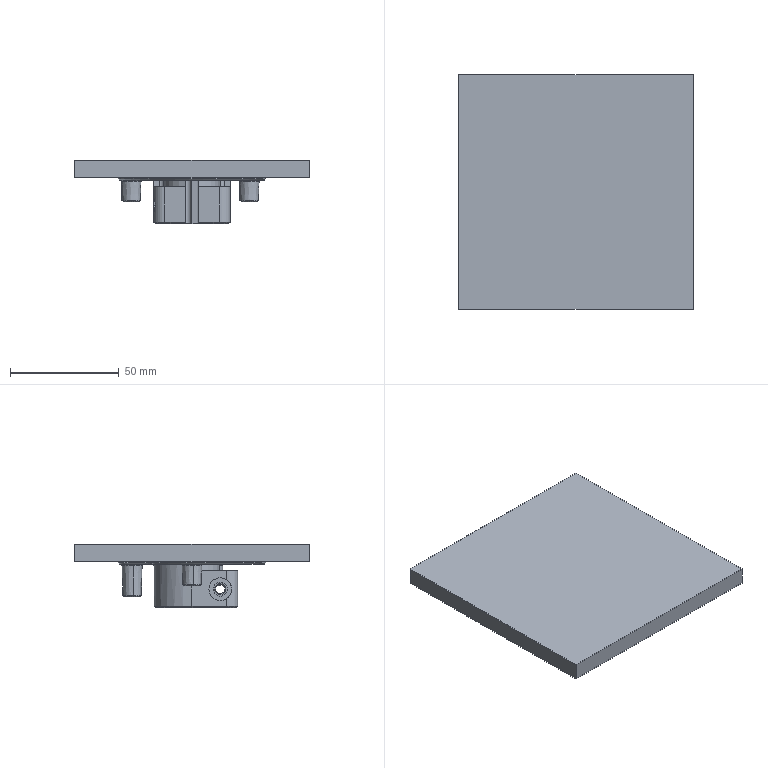NC program | NX | posted with a generic post | part box 108 x 108 x 29 mm
Lines 5403 to 6183 of 23883:
(ZLEVEL_PROFILE_COPY_COPY_COPY_COPY_1 , TOOL : D3R0.5)
N10768 T07 M6
N10770 G54
N10772 G17 G0 G90 X-0.847 Y24.584 S9500 M3
N10774 G43 Z30. H7
N10776 Z-4.
N10778 G94 G1 X-1.263 Y24.078 Z-4.034 F1000.
N10780 X-1.883 Y23.537 Z-4.077
N10782 X-2.582 Y23.105 Z-4.121
N10784 X-3.342 Y22.793 Z-4.164
N10786 X-4.144 Y22.608 Z-4.207
N10788 X-4.964 Y22.558 Z-4.25
N10790 X-5.782 Y22.642 Z-4.293
N10792 X-6.575 Y22.858 Z-4.336
N10794 X-7.322 Y23.201 Z-4.379
N10796 X-8.003 Y23.661 Z-4.422
N10798 X-8.6 Y24.227 Z-4.465
N10800 X-8.992 Y24.724 Z-4.498
N10802 X-9.402 Y25.437 Z-4.541
N10804 X-9.691 Y26.206 Z-4.585
N10806 X-9.849 Y27.013 Z-4.628
N10808 X-9.874 Y27.835 Z-4.671
N10810 X-9.764 Y28.65 Z-4.714
N10812 X-9.523 Y29.436 Z-4.757
N10814 X-9.157 Y30.172 Z-4.8
N10816 X-8.675 Y30.838 Z-4.843
N10818 X-8.091 Y31.417 Z-4.886
N10820 X-7.421 Y31.892 Z-4.929
N10822 X-6.681 Y32.252 Z-4.972
N10824 X-5.893 Y32.486 Z-5.015
N10826 X-5.267 Y32.577 Z-5.049
N10828 X-5.179 Y32.583 Z-5.053
N10830 X-4.863 Z-5.07
N10832 G2 X0.146 Y27.575 R5.008 F2000.
N10834 X-4.863 Y32.583 R-5.008
N10836 G1 X-4.745 Y32.579 Z-5.072
N10838 X-4.627 Y32.577 Z-5.074
N10840 X-4.51 Y32.575 Z-5.076
N10842 X-4.392 Y32.573 Z-5.078
N10844 X-4.274 Y32.563 Z-5.08
N10846 X-4.158 Y32.545 Z-5.082
N10848 X-4.041 Y32.53 Z-5.084
N10850 X-3.924 Y32.513 Z-5.086
N10852 X-3.808 Y32.492 Z-5.088
N10854 X-3.691 Y32.472 Z-5.09
N10856 X-3.576 Y32.444 Z-5.092
N10858 X-3.462 Y32.414 Z-5.094
N10860 X-3.348 Y32.383 Z-5.096
N10862 X-3.235 Y32.348 Z-5.099
N10864 X-3.122 Y32.311 Z-5.101
N10866 X-3.01 Y32.273 Z-5.103
N10868 X-2.899 Y32.229 Z-5.105
N10870 X-2.79 Y32.185 Z-5.107
N10872 X-2.681 Y32.137 Z-5.109
N10874 X-2.573 Y32.087 Z-5.111
N10876 X-2.467 Y32.034 Z-5.113
N10878 X-2.361 Y31.979 Z-5.115
N10880 X-2.258 Y31.921 Z-5.117
N10882 X-2.155 Y31.861 Z-5.119
N10884 X-2.054 Y31.798 Z-5.121
N10886 X-1.954 Y31.733 Z-5.123
N10888 X-1.856 Y31.665 Z-5.125
N10890 X-1.759 Y31.595 Z-5.127
N10892 X-1.664 Y31.523 Z-5.129
N10894 X-1.571 Y31.449 Z-5.131
N10896 X-1.479 Y31.372 Z-5.133
N10898 X-1.39 Y31.293 Z-5.135
N10900 X-1.302 Y31.212 Z-5.138
N10902 X-1.216 Y31.129 Z-5.14
N10904 G2 X-4.863 Y32.667 R-5.092
N10906 G1 X-4.745 Y32.668 Z-5.142
N10908 X-4.627 Y32.666 Z-5.144
N10910 X-4.51 Y32.661 Z-5.146
N10912 X-4.392 Y32.653 Z-5.148
N10914 X-4.275 Y32.643 Z-5.15
N10916 X-4.158 Y32.631 Z-5.152
N10918 X-4.041 Y32.615 Z-5.154
N10920 X-3.924 Y32.597 Z-5.156
N10922 X-3.808 Y32.576 Z-5.158
N10924 X-3.692 Y32.552 Z-5.16
N10926 X-3.577 Y32.526 Z-5.162
N10928 X-3.463 Y32.497 Z-5.164
N10930 X-3.349 Y32.465 Z-5.166
N10932 X-3.236 Y32.431 Z-5.168
N10934 X-3.123 Y32.394 Z-5.17
N10936 X-3.012 Y32.355 Z-5.172
N10938 X-2.901 Y32.313 Z-5.174
N10940 X-2.791 Y32.268 Z-5.177
N10942 X-2.682 Y32.221 Z-5.179
N10944 X-2.575 Y32.171 Z-5.181
N10946 X-2.468 Y32.119 Z-5.183
N10948 X-2.363 Y32.064 Z-5.185
N10950 X-2.259 Y32.007 Z-5.187
N10952 X-2.156 Y31.948 Z-5.189
N10954 X-2.055 Y31.886 Z-5.191
N10956 X-1.955 Y31.822 Z-5.193
N10958 X-1.856 Y31.755 Z-5.195
N10960 X-1.759 Y31.686 Z-5.197
N10962 X-1.664 Y31.615 Z-5.199
N10964 X-1.57 Y31.542 Z-5.201
N10966 X-1.478 Y31.467 Z-5.203
N10968 X-1.388 Y31.389 Z-5.205
N10970 X-1.299 Y31.309 Z-5.207
N10972 X-1.212 Y31.227 Z-5.209
N10974 G2 X-4.863 Y32.738 R-5.164
N10976 G1 X-4.745 Y32.739 Z-5.211
N10978 X-4.627 Y32.737 Z-5.213
N10980 X-4.51 Y32.733 Z-5.215
N10982 X-4.392 Y32.725 Z-5.218
N10984 X-4.275 Y32.715 Z-5.22
N10986 X-4.158 Y32.703 Z-5.222
N10988 X-4.041 Y32.688 Z-5.224
N10990 X-3.924 Y32.67 Z-5.226
N10992 X-3.808 Y32.649 Z-5.228
N10994 X-3.692 Y32.626 Z-5.23
N10996 X-3.577 Y32.6 Z-5.232
N10998 X-3.462 Y32.571 Z-5.234
N11000 X-3.348 Y32.54 Z-5.236
N11002 X-3.235 Y32.506 Z-5.238
N11004 X-3.122 Y32.47 Z-5.24
N11006 X-3.011 Y32.431 Z-5.242
N11008 X-2.9 Y32.39 Z-5.244
N11010 X-2.79 Y32.346 Z-5.246
N11012 X-2.681 Y32.299 Z-5.248
N11014 X-2.573 Y32.25 Z-5.25
N11016 X-2.466 Y32.199 Z-5.252
N11018 X-2.36 Y32.145 Z-5.254
N11020 X-2.256 Y32.088 Z-5.257
N11022 X-2.153 Y32.03 Z-5.259
N11024 X-2.051 Y31.969 Z-5.261
N11026 X-1.95 Y31.905 Z-5.263
N11028 X-1.851 Y31.84 Z-5.265
N11030 X-1.754 Y31.772 Z-5.267
N11032 X-1.658 Y31.701 Z-5.269
N11034 X-1.563 Y31.629 Z-5.271
N11036 X-1.47 Y31.554 Z-5.273
N11038 X-1.379 Y31.478 Z-5.275
N11040 X-1.29 Y31.399 Z-5.277
N11042 X-1.202 Y31.318 Z-5.279
N11044 G2 X-4.863 Y32.81 R-5.235
N11046 G1 X-4.745 Y32.811 Z-5.281
N11048 X-4.627 Y32.809 Z-5.283
N11050 X-4.51 Y32.804 Z-5.285
N11052 X-4.392 Y32.797 Z-5.287
N11054 X-4.275 Y32.788 Z-5.289
N11056 X-4.158 Y32.775 Z-5.291
N11058 X-4.041 Y32.76 Z-5.293
N11060 X-3.924 Y32.742 Z-5.296
N11062 X-3.808 Y32.722 Z-5.298
N11064 X-3.692 Y32.699 Z-5.3
N11066 X-3.577 Y32.674 Z-5.302
N11068 X-3.462 Y32.646 Z-5.304
N11070 X-3.348 Y32.615 Z-5.306
N11072 X-3.234 Y32.582 Z-5.308
N11074 X-3.122 Y32.546 Z-5.31
N11076 X-3.01 Y32.507 Z-5.312
N11078 X-2.899 Y32.466 Z-5.314
N11080 X-2.788 Y32.423 Z-5.316
N11082 X-2.679 Y32.377 Z-5.318
N11084 X-2.571 Y32.329 Z-5.32
N11086 X-2.464 Y32.278 Z-5.322
N11088 X-2.358 Y32.225 Z-5.324
N11090 X-2.253 Y32.169 Z-5.326
N11092 X-2.149 Y32.111 Z-5.328
N11094 X-2.047 Y32.051 Z-5.33
N11096 X-1.946 Y31.989 Z-5.332
N11098 X-1.846 Y31.924 Z-5.335
N11100 X-1.748 Y31.857 Z-5.337
N11102 X-1.652 Y31.787 Z-5.339
N11104 X-1.557 Y31.716 Z-5.341
N11106 X-1.463 Y31.642 Z-5.343
N11108 X-1.371 Y31.566 Z-5.345
N11110 X-1.281 Y31.488 Z-5.347
N11112 X-1.193 Y31.409 Z-5.349
N11114 G2 X-4.863 Y32.882 R-5.307
N11116 G1 X-4.745 Z-5.351
N11118 X-4.627 Y32.881 Z-5.353
N11120 X-4.51 Y32.876 Z-5.355
N11122 X-4.392 Y32.869 Z-5.357
N11124 X-4.275 Y32.86 Z-5.359
N11126 X-4.157 Y32.847 Z-5.361
N11128 X-4.04 Y32.833 Z-5.363
N11130 X-3.924 Y32.815 Z-5.365
N11132 X-3.808 Y32.795 Z-5.367
N11134 X-3.692 Y32.773 Z-5.369
N11136 X-3.576 Y32.747 Z-5.371
N11138 X-3.462 Y32.72 Z-5.374
N11140 X-3.347 Y32.689 Z-5.376
N11142 X-3.234 Y32.657 Z-5.378
N11144 X-3.121 Y32.621 Z-5.38
N11146 X-3.009 Y32.583 Z-5.382
N11148 X-2.897 Y32.543 Z-5.384
N11150 X-2.787 Y32.5 Z-5.386
N11152 X-2.678 Y32.455 Z-5.388
N11154 X-2.569 Y32.407 Z-5.39
N11156 X-2.462 Y32.357 Z-5.392
N11158 X-2.355 Y32.305 Z-5.394
N11160 X-2.25 Y32.25 Z-5.396
N11162 X-2.146 Y32.193 Z-5.398
N11164 X-2.043 Y32.133 Z-5.4
N11166 X-1.942 Y32.071 Z-5.402
N11168 X-1.842 Y32.007 Z-5.404
N11170 X-1.743 Y31.941 Z-5.406
N11172 X-1.646 Y31.873 Z-5.408
N11174 X-1.55 Y31.802 Z-5.41
N11176 X-1.456 Y31.729 Z-5.413
N11178 X-1.363 Y31.654 Z-5.415
N11180 X-1.272 Y31.577 Z-5.417
N11182 X-1.183 Y31.498 Z-5.419
N11184 G2 X-4.863 Y32.953 R-5.379
N11186 G1 X-4.745 Y32.954 Z-5.421
N11188 X-4.627 Y32.952 Z-5.423
N11190 X-4.51 Y32.948 Z-5.425
N11192 X-4.392 Y32.941 Z-5.427
N11194 X-4.275 Y32.932 Z-5.429
N11196 X-4.157 Y32.92 Z-5.431
N11198 X-4.04 Y32.905 Z-5.433
N11200 X-3.924 Y32.888 Z-5.435
N11202 X-3.807 Y32.868 Z-5.437
N11204 X-3.692 Y32.846 Z-5.439
N11206 X-3.576 Y32.821 Z-5.441
N11208 X-3.461 Y32.794 Z-5.443
N11210 X-3.347 Y32.764 Z-5.445
N11212 X-3.233 Y32.732 Z-5.447
N11214 X-3.12 Y32.697 Z-5.449
N11216 X-3.008 Y32.659 Z-5.452
N11218 X-2.896 Y32.62 Z-5.454
N11220 X-2.786 Y32.577 Z-5.456
N11222 X-2.676 Y32.533 Z-5.458
N11224 X-2.567 Y32.486 Z-5.46
N11226 X-2.46 Y32.436 Z-5.462
N11228 X-2.353 Y32.384 Z-5.464
N11230 X-2.247 Y32.33 Z-5.466
N11232 X-2.143 Y32.274 Z-5.468
N11234 X-2.04 Y32.215 Z-5.47
N11236 X-1.938 Y32.154 Z-5.472
N11238 X-1.837 Y32.091 Z-5.474
N11240 X-1.738 Y32.025 Z-5.476
N11242 X-1.64 Y31.958 Z-5.478
N11244 X-1.544 Y31.888 Z-5.48
N11246 X-1.449 Y31.816 Z-5.482
N11248 X-1.356 Y31.742 Z-5.484
N11250 X-1.264 Y31.666 Z-5.486
N11252 X-1.174 Y31.588 Z-5.488
N11254 G2 X-4.863 Y33.025 R-5.45
N11256 G1 X-4.745 Y33.026 Z-5.491
N11258 X-4.627 Y33.024 Z-5.493
N11260 X-4.51 Y33.02 Z-5.495
N11262 X-4.392 Y33.013 Z-5.497
N11264 X-4.275 Y33.004 Z-5.499
N11266 X-4.157 Y32.992 Z-5.501
N11268 X-4.04 Y32.978 Z-5.503
N11270 X-3.924 Y32.961 Z-5.505
N11272 X-3.807 Y32.941 Z-5.507
N11274 X-3.691 Y32.919 Z-5.509
N11276 X-3.576 Y32.895 Z-5.511
N11278 X-3.461 Y32.868 Z-5.513
N11280 X-3.346 Y32.838 Z-5.515
N11282 X-3.233 Y32.807 Z-5.517
N11284 X-3.119 Y32.772 Z-5.519
N11286 X-3.007 Y32.735 Z-5.521
N11288 X-2.895 Y32.696 Z-5.523
N11290 X-2.785 Y32.654 Z-5.525
N11292 X-2.675 Y32.61 Z-5.527
N11294 X-2.566 Y32.564 Z-5.53
N11296 X-2.458 Y32.515 Z-5.532
N11298 X-2.351 Y32.464 Z-5.534
N11300 X-2.245 Y32.41 Z-5.536
N11302 X-2.14 Y32.355 Z-5.538
N11304 X-2.036 Y32.297 Z-5.54
N11306 X-1.934 Y32.236 Z-5.542
N11308 X-1.833 Y32.174 Z-5.544
N11310 X-1.733 Y32.109 Z-5.546
N11312 X-1.635 Y32.042 Z-5.548
N11314 X-1.538 Y31.973 Z-5.55
N11316 X-1.443 Y31.902 Z-5.552
N11318 X-1.349 Y31.829 Z-5.554
N11320 X-1.256 Y31.754 Z-5.556
N11322 X-1.166 Y31.677 Z-5.558
N11324 G2 X-4.863 Y33.097 R-5.522
N11326 G1 X-4.745 Z-5.56
N11328 X-4.627 Y33.096 Z-5.562
N11330 X-4.51 Y33.092 Z-5.564
N11332 X-4.392 Y33.085 Z-5.566
N11334 X-4.275 Y33.076 Z-5.568
N11336 X-4.157 Y33.064 Z-5.571
N11338 X-4.04 Y33.05 Z-5.573
N11340 X-3.924 Y33.033 Z-5.575
N11342 X-3.807 Y33.014 Z-5.577
N11344 X-3.691 Y32.993 Z-5.579
N11346 X-3.576 Y32.968 Z-5.581
N11348 X-3.461 Y32.942 Z-5.583
N11350 X-3.346 Y32.913 Z-5.585
N11352 X-3.232 Y32.881 Z-5.587
N11354 X-3.119 Y32.847 Z-5.589
N11356 X-3.006 Y32.811 Z-5.591
N11358 X-2.894 Y32.772 Z-5.593
N11360 X-2.783 Y32.731 Z-5.595
N11362 X-2.673 Y32.688 Z-5.597
N11364 X-2.564 Y32.642 Z-5.599
N11366 X-2.456 Y32.594 Z-5.601
N11368 X-2.348 Y32.543 Z-5.603
N11370 X-2.242 Y32.49 Z-5.605
N11372 X-2.137 Y32.435 Z-5.607
N11374 X-2.033 Y32.378 Z-5.61
N11376 X-1.93 Y32.319 Z-5.612
N11378 X-1.829 Y32.257 Z-5.614
N11380 X-1.729 Y32.193 Z-5.616
N11382 X-1.63 Y32.127 Z-5.618
N11384 X-1.533 Y32.059 Z-5.62
N11386 X-1.436 Y31.988 Z-5.622
N11388 X-1.342 Y31.916 Z-5.624
N11390 X-1.249 Y31.842 Z-5.626
N11392 X-1.158 Y31.766 Z-5.628
N11394 G2 X-4.863 Y33.168 R-5.594
N11396 G1 X-4.744 Y33.169 Z-5.63
N11398 X-4.626 Y33.167 Z-5.632
N11400 X-4.508 Y33.163 Z-5.634
N11402 X-4.39 Y33.157 Z-5.636
N11404 X-4.272 Y33.148 Z-5.638
N11406 X-4.154 Y33.136 Z-5.64
N11408 X-4.036 Y33.122 Z-5.642
N11410 X-3.919 Y33.105 Z-5.645
N11412 X-3.802 Y33.086 Z-5.647
N11414 X-3.685 Y33.065 Z-5.649
N11416 X-3.569 Y33.04 Z-5.651
N11418 X-3.453 Y33.014 Z-5.653
N11420 X-3.338 Y32.985 Z-5.655
N11422 X-3.223 Y32.953 Z-5.657
N11424 X-3.109 Y32.919 Z-5.659
N11426 X-2.996 Y32.883 Z-5.661
N11428 X-2.884 Y32.844 Z-5.663
N11430 X-2.772 Y32.803 Z-5.665
N11432 X-2.661 Y32.759 Z-5.667
N11434 X-2.552 Y32.713 Z-5.669
N11436 X-2.443 Y32.665 Z-5.671
N11438 X-2.335 Y32.615 Z-5.673
N11440 X-2.228 Y32.562 Z-5.675
N11442 X-2.122 Y32.506 Z-5.678
N11444 X-2.018 Y32.449 Z-5.68
N11446 X-1.915 Y32.389 Z-5.682
N11448 X-1.813 Y32.327 Z-5.684
N11450 X-1.712 Y32.263 Z-5.686
N11452 X-1.613 Y32.197 Z-5.688
N11454 X-1.515 Y32.129 Z-5.69
N11456 X-1.418 Y32.058 Z-5.692
N11458 X-1.323 Y31.986 Z-5.694
N11460 X-1.23 Y31.911 Z-5.696
N11462 X-1.138 Y31.835 Z-5.698
N11464 X-1.048 Y31.756 Z-5.7
N11466 X-0.959 Y31.676 Z-5.702
N11468 G2 X-4.863 Y33.236 R-5.662
N11470 G1 X-4.745 Y33.237 Z-5.704
N11472 X-4.628 Y33.235 Z-5.706
N11474 X-4.511 Y33.23 Z-5.708
N11476 X-4.394 Y33.223 Z-5.71
N11478 X-4.277 Y33.214 Z-5.713
N11480 X-4.161 Y33.202 Z-5.715
N11482 X-4.044 Y33.188 Z-5.717
N11484 X-3.928 Y33.171 Z-5.719
N11486 X-3.812 Y33.152 Z-5.721
N11488 X-3.697 Y33.13 Z-5.723
N11490 X-3.582 Y33.106 Z-5.725
N11492 X-3.468 Y33.08 Z-5.727
N11494 X-3.354 Y33.051 Z-5.729
N11496 X-3.241 Y33.02 Z-5.731
N11498 X-3.128 Y32.987 Z-5.733
N11500 X-3.016 Y32.951 Z-5.735
N11502 X-2.905 Y32.913 Z-5.737
N11504 X-2.794 Y32.872 Z-5.739
N11506 X-2.685 Y32.83 Z-5.741
N11508 X-2.576 Y32.785 Z-5.743
N11510 X-2.468 Y32.737 Z-5.745
N11512 X-2.361 Y32.688 Z-5.747
N11514 X-2.256 Y32.636 Z-5.749
N11516 X-2.151 Y32.582 Z-5.751
N11518 X-2.047 Y32.526 Z-5.753
N11520 X-1.945 Y32.468 Z-5.755
N11522 X-1.844 Y32.408 Z-5.757
N11524 X-1.744 Y32.345 Z-5.76
N11526 X-1.645 Y32.281 Z-5.762
N11528 X-1.548 Y32.214 Z-5.764
N11530 X-1.452 Y32.145 Z-5.766
N11532 X-1.358 Y32.075 Z-5.768
N11534 X-1.265 Y32.002 Z-5.77
N11536 X-1.173 Y31.928 Z-5.772
N11538 X-1.083 Y31.851 Z-5.774
N11540 X-0.995 Y31.773 Z-5.776
N11542 X-0.908 Y31.693 Z-5.778
N11544 X-0.823 Y31.611 Z-5.78
N11546 X-0.74 Y31.527 Z-5.782
N11548 X-0.658 Y31.442 Z-5.784
N11550 X-0.579 Y31.355 Z-5.786
N11552 X-0.501 Y31.266 Z-5.788
N11554 G2 X-4.863 Y33.289 R-5.714
N11556 G1 X-4.745 Y33.288 Z-5.79
N11558 X-4.628 Y33.286 Z-5.792
N11560 X-4.51 Y33.281 Z-5.794
N11562 X-4.393 Y33.273 Z-5.796
N11564 X-4.276 Y33.263 Z-5.798
N11566 X-4.159 Y33.251 Z-5.8
N11568 X-4.043 Y33.236 Z-5.802
N11570 X-3.926 Y33.219 Z-5.805
N11572 X-3.811 Y33.2 Z-5.807
N11574 X-3.695 Y33.178 Z-5.809
N11576 X-3.58 Y33.153 Z-5.811
N11578 X-3.465 Y33.127 Z-5.813
N11580 X-3.351 Y33.098 Z-5.815
N11582 X-3.238 Y33.066 Z-5.817
N11584 X-3.125 Y33.033 Z-5.819
N11586 X-3.013 Y32.996 Z-5.821
N11588 X-2.902 Y32.958 Z-5.823
N11590 X-2.792 Y32.917 Z-5.825
N11592 X-2.682 Y32.874 Z-5.827
N11594 X-2.573 Y32.829 Z-5.829
N11596 X-2.465 Y32.782 Z-5.831
N11598 X-2.359 Y32.732 Z-5.833
N11600 X-2.253 Y32.68 Z-5.835
N11602 X-2.148 Y32.626 Z-5.837
N11604 X-2.045 Y32.57 Z-5.839
N11606 X-1.942 Y32.512 Z-5.841
N11608 X-1.841 Y32.451 Z-5.843
N11610 X-1.741 Y32.389 Z-5.845
N11612 X-1.643 Y32.324 Z-5.848
N11614 X-1.545 Y32.258 Z-5.85
N11616 X-1.449 Y32.189 Z-5.852
N11618 X-1.355 Y32.119 Z-5.854
N11620 X-1.262 Y32.046 Z-5.856
N11622 X-1.17 Y31.972 Z-5.858
N11624 X-1.081 Y31.895 Z-5.86
N11626 X-0.992 Y31.817 Z-5.862
N11628 X-0.905 Y31.737 Z-5.864
N11630 X-0.82 Y31.656 Z-5.866
N11632 X-0.737 Y31.572 Z-5.868
N11634 X-0.655 Y31.487 Z-5.87
N11636 X-0.575 Y31.4 Z-5.872
N11638 X-0.497 Y31.311 Z-5.874
N11640 X-0.421 Y31.221 Z-5.876
N11642 X-0.347 Y31.13 Z-5.878
N11644 X-0.274 Y31.036 Z-5.88
N11646 X-0.203 Y30.942 Z-5.882
N11648 G2 X-4.863 Y33.323 R-5.748
N11650 G1 X-4.745 Y33.322 Z-5.884
N11652 X-4.627 Y33.319 Z-5.886
N11654 X-4.509 Y33.313 Z-5.889
N11656 X-4.391 Y33.305 Z-5.891
N11658 X-4.273 Y33.295 Z-5.893
N11660 X-4.156 Y33.282 Z-5.895
N11662 X-4.039 Y33.267 Z-5.897
N11664 X-3.922 Y33.249 Z-5.899
N11666 X-3.805 Y33.229 Z-5.901
N11668 X-3.689 Y33.207 Z-5.903
N11670 X-3.574 Y33.182 Z-5.905
N11672 X-3.459 Y33.155 Z-5.907
N11674 X-3.345 Y33.125 Z-5.909
N11676 X-3.231 Y33.093 Z-5.911
N11678 X-3.118 Y33.059 Z-5.913
N11680 X-3.005 Y33.022 Z-5.915
N11682 X-2.894 Y32.983 Z-5.917
N11684 X-2.783 Y32.942 Z-5.919
N11686 X-2.673 Y32.898 Z-5.922
N11688 X-2.564 Y32.853 Z-5.924
N11690 X-2.456 Y32.805 Z-5.926
N11692 X-2.349 Y32.754 Z-5.928
N11694 X-2.243 Y32.702 Z-5.93
N11696 X-2.138 Y32.647 Z-5.932
N11698 X-2.034 Y32.591 Z-5.934
N11700 X-1.932 Y32.532 Z-5.936
N11702 X-1.831 Y32.471 Z-5.938
N11704 X-1.731 Y32.408 Z-5.94
N11706 X-1.632 Y32.343 Z-5.942
N11708 X-1.534 Y32.276 Z-5.944
N11710 X-1.438 Y32.206 Z-5.946
N11712 X-1.344 Y32.135 Z-5.948
N11714 X-1.251 Y32.062 Z-5.95
N11716 X-1.159 Y31.987 Z-5.952
N11718 X-1.069 Y31.911 Z-5.954
N11720 X-0.981 Y31.832 Z-5.957
N11722 X-0.894 Y31.751 Z-5.959
N11724 X-0.809 Y31.669 Z-5.961
N11726 X-0.726 Y31.585 Z-5.963
N11728 X-0.644 Y31.5 Z-5.965
N11730 X-0.564 Y31.412 Z-5.967
N11732 X-0.486 Y31.323 Z-5.969
N11734 X-0.41 Y31.233 Z-5.971
N11736 X-0.336 Y31.141 Z-5.973
N11738 X-0.264 Y31.047 Z-5.975
N11740 X-0.193 Y30.952 Z-5.977
N11742 X-0.125 Y30.855 Z-5.979
N11744 X-0.058 Y30.758 Z-5.981
N11746 G2 X-1.572 Y22.844 R5.763
N11748 G1 X-1.749 Y22.725
N11750 G2 X-5.177 Y21.821 R5.763
N11752 G1 X-5.441 Y21.841
N11754 G2 X-9.975 Y24.916 R5.763
N11756 G1 X-10.014 Y24.993
N11758 G2 X-10.201 Y25.405 R5.763
N11760 G1 X-10.262 Y25.563
N11762 G2 X-10.498 Y26.373 R5.763
N11764 G1 X-10.507 Y26.414
N11766 G2 X-4.863 Y33.337 R5.763
N11768 G1 X-4.743 Y33.336 Z-5.983
N11770 X-4.624 Y33.333 Z-5.985
N11772 X-4.505 Y33.326 Z-5.988
N11774 X-4.386 Y33.318 Z-5.99
N11776 X-4.267 Y33.307 Z-5.992
N11778 X-4.149 Y33.293 Z-5.994
N11780 X-4.03 Y33.277 Z-5.996
N11782 X-3.912 Y33.259 Z-5.998
N11784 X-3.795 Y33.238 Z-6.
N11786 X-3.678 Y33.215 Z-6.002
N11788 X-3.561 Y33.189 Z-6.004
N11790 X-3.445 Y33.161 Z-6.006
N11792 X-3.33 Y33.131 Z-6.008
N11794 X-3.215 Y33.098 Z-6.01
N11796 X-3.101 Y33.063 Z-6.013
N11798 X-2.988 Y33.025 Z-6.015
N11800 X-2.876 Y32.985 Z-6.017
N11802 X-2.764 Y32.943 Z-6.019
N11804 X-2.653 Y32.898 Z-6.021
N11806 X-2.544 Y32.852 Z-6.023
N11808 X-2.435 Y32.803 Z-6.025
N11810 X-2.327 Y32.751 Z-6.027
N11812 X-2.22 Y32.698 Z-6.029
N11814 X-2.115 Y32.642 Z-6.031
N11816 X-2.011 Y32.584 Z-6.033
N11818 X-1.907 Y32.524 Z-6.035
N11820 X-1.806 Y32.462 Z-6.037
N11822 X-1.705 Y32.397 Z-6.04
N11824 X-1.606 Y32.331 Z-6.042
N11826 X-1.508 Y32.263 Z-6.044
N11828 X-1.412 Y32.192 Z-6.046
N11830 X-1.317 Y32.12 Z-6.048
N11832 X-1.223 Y32.046 Z-6.05
N11834 X-1.132 Y31.969 Z-6.052
N11836 X-1.041 Y31.891 Z-6.054
N11838 X-0.953 Y31.811 Z-6.056
N11840 X-0.866 Y31.73 Z-6.058
N11842 X-0.781 Y31.646 Z-6.06
N11844 X-0.697 Y31.561 Z-6.062
N11846 X-0.616 Y31.474 Z-6.065
N11848 X-0.536 Y31.385 Z-6.067
N11850 X-0.458 Y31.295 Z-6.069
N11852 X-0.382 Y31.203 Z-6.071
N11854 X-0.308 Y31.109 Z-6.073
N11856 X-0.235 Y31.014 Z-6.075
N11858 X-0.165 Y30.918 Z-6.077
N11860 X-0.097 Y30.82 Z-6.079
N11862 X-0.031 Y30.72 Z-6.081
N11864 G2 X-4.863 Y33.34 R-5.765
N11866 G1 X-4.743 Y33.339 Z-6.083
N11868 X-4.624 Y33.335 Z-6.085
N11870 X-4.505 Y33.329 Z-6.087
N11872 X-4.386 Y33.321 Z-6.09
N11874 X-4.267 Y33.309 Z-6.092
N11876 X-4.149 Y33.296 Z-6.094
N11878 X-4.03 Y33.28 Z-6.096
N11880 X-3.912 Y33.262 Z-6.098
N11882 X-3.795 Y33.241 Z-6.1
N11884 X-3.678 Y33.218 Z-6.102
N11886 X-3.561 Y33.192 Z-6.104
N11888 X-3.445 Y33.164 Z-6.106
N11890 X-3.33 Y33.133 Z-6.108
N11892 X-3.215 Y33.101 Z-6.11
N11894 X-3.101 Y33.065 Z-6.112
N11896 X-2.988 Y33.028 Z-6.115
N11898 X-2.875 Y32.988 Z-6.117
N11900 X-2.764 Y32.946 Z-6.119
N11902 X-2.653 Y32.901 Z-6.121
N11904 X-2.543 Y32.854 Z-6.123
N11906 X-2.435 Y32.805 Z-6.125
N11908 X-2.327 Y32.754 Z-6.127
N11910 X-2.22 Y32.7 Z-6.129
N11912 X-2.115 Y32.645 Z-6.131
N11914 X-2.01 Y32.587 Z-6.133
N11916 X-1.907 Y32.527 Z-6.135
N11918 X-1.805 Y32.465 Z-6.137
N11920 X-1.705 Y32.4 Z-6.14
N11922 X-1.606 Y32.334 Z-6.142
N11924 X-1.508 Y32.266 Z-6.144
N11926 X-1.411 Y32.195 Z-6.146
N11928 X-1.316 Y32.123 Z-6.148
N11930 X-1.223 Y32.049 Z-6.15
N11932 X-1.131 Y31.972 Z-6.152
N11934 X-1.041 Y31.894 Z-6.154
N11936 X-0.952 Y31.814 Z-6.156
N11938 X-0.865 Y31.733 Z-6.158
N11940 X-0.78 Y31.649 Z-6.16
N11942 X-0.697 Y31.564 Z-6.162
N11944 X-0.615 Y31.477 Z-6.165
N11946 X-0.535 Y31.388 Z-6.167
N11948 X-0.457 Y31.298 Z-6.169
N11950 X-0.381 Y31.206 Z-6.171
N11952 X-0.307 Y31.112 Z-6.173
N11954 X-0.234 Y31.017 Z-6.175
N11956 X-0.164 Y30.921 Z-6.177
N11958 X-0.096 Y30.823 Z-6.179
N11960 X-0.03 Y30.724 Z-6.181
N11962 G2 X-4.863 Y33.343 R-5.768
N11964 G1 X-4.743 Y33.341 Z-6.183
N11966 X-4.624 Y33.338 Z-6.185
N11968 X-4.505 Y33.332 Z-6.187
N11970 X-4.386 Y33.323 Z-6.19
N11972 X-4.267 Y33.312 Z-6.192
N11974 X-4.148 Y33.299 Z-6.194
N11976 X-4.03 Y33.283 Z-6.196
N11978 X-3.912 Y33.264 Z-6.198
N11980 X-3.795 Y33.244 Z-6.2
N11982 X-3.678 Y33.22 Z-6.202
N11984 X-3.561 Y33.195 Z-6.204
N11986 X-3.445 Y33.167 Z-6.206
N11988 X-3.33 Y33.136 Z-6.208
N11990 X-3.215 Y33.103 Z-6.21
N11992 X-3.101 Y33.068 Z-6.212
N11994 X-2.988 Y33.031 Z-6.215
N11996 X-2.875 Y32.991 Z-6.217
N11998 X-2.764 Y32.948 Z-6.219
N12000 X-2.653 Y32.904 Z-6.221
N12002 X-2.543 Y32.857 Z-6.223
N12004 X-2.435 Y32.808 Z-6.225
N12006 X-2.327 Y32.757 Z-6.227
N12008 X-2.22 Y32.703 Z-6.229
N12010 X-2.115 Y32.648 Z-6.231
N12012 X-2.01 Y32.59 Z-6.233
N12014 X-1.907 Y32.53 Z-6.235
N12016 X-1.805 Y32.468 Z-6.237
N12018 X-1.705 Y32.403 Z-6.24
N12020 X-1.605 Y32.337 Z-6.242
N12022 X-1.508 Y32.269 Z-6.244
N12024 X-1.411 Y32.198 Z-6.246
N12026 X-1.316 Y32.126 Z-6.248
N12028 X-1.223 Y32.052 Z-6.25
N12030 X-1.131 Y31.976 Z-6.252
N12032 X-1.041 Y31.898 Z-6.254
N12034 X-0.952 Y31.818 Z-6.256
N12036 X-0.865 Y31.736 Z-6.258
N12038 X-0.78 Y31.652 Z-6.26
N12040 X-0.696 Y31.567 Z-6.262
N12042 X-0.615 Y31.48 Z-6.265
N12044 X-0.535 Y31.391 Z-6.267
N12046 X-0.457 Y31.301 Z-6.269
N12048 X-0.38 Y31.209 Z-6.271
N12050 X-0.306 Y31.116 Z-6.273
N12052 X-0.234 Y31.021 Z-6.275
N12054 X-0.163 Y30.924 Z-6.277
N12056 X-0.095 Y30.827 Z-6.279
N12058 X-0.029 Y30.727 Z-6.281
N12060 G2 X-4.863 Y33.345 R-5.771
N12062 G1 X-4.743 Y33.344 Z-6.283
N12064 X-4.624 Y33.34 Z-6.285
N12066 X-4.505 Y33.334 Z-6.287
N12068 X-4.386 Y33.326 Z-6.289
N12070 X-4.267 Y33.315 Z-6.292
N12072 X-4.148 Y33.301 Z-6.294
N12074 X-4.03 Y33.285 Z-6.296
N12076 X-3.912 Y33.267 Z-6.298
N12078 X-3.795 Y33.246 Z-6.3
N12080 X-3.678 Y33.223 Z-6.302
N12082 X-3.561 Y33.197 Z-6.304
N12084 X-3.445 Y33.169 Z-6.306
N12086 X-3.33 Y33.139 Z-6.308
N12088 X-3.215 Y33.106 Z-6.31
N12090 X-3.101 Y33.071 Z-6.312
N12092 X-2.988 Y33.033 Z-6.314
N12094 X-2.875 Y32.993 Z-6.317
N12096 X-2.764 Y32.951 Z-6.319
N12098 X-2.653 Y32.907 Z-6.321
N12100 X-2.543 Y32.86 Z-6.323
N12102 X-2.434 Y32.811 Z-6.325
N12104 X-2.327 Y32.76 Z-6.327
N12106 X-2.22 Y32.706 Z-6.329
N12108 X-2.114 Y32.651 Z-6.331
N12110 X-2.01 Y32.593 Z-6.333
N12112 X-1.907 Y32.533 Z-6.335
N12114 X-1.805 Y32.471 Z-6.337
N12116 X-1.704 Y32.406 Z-6.339
N12118 X-1.605 Y32.34 Z-6.342
N12120 X-1.507 Y32.272 Z-6.344
N12122 X-1.411 Y32.202 Z-6.346
N12124 X-1.316 Y32.129 Z-6.348
N12126 X-1.222 Y32.055 Z-6.35
N12128 X-1.131 Y31.979 Z-6.352
N12130 X-1.04 Y31.901 Z-6.354
N12132 X-0.952 Y31.821 Z-6.356
N12134 X-0.865 Y31.739 Z-6.358
N12136 X-0.779 Y31.656 Z-6.36
N12138 X-0.696 Y31.57 Z-6.362
N12140 X-0.614 Y31.483 Z-6.364
N12142 X-0.534 Y31.395 Z-6.367
N12144 X-0.456 Y31.305 Z-6.369
N12146 X-0.38 Y31.213 Z-6.371
N12148 X-0.306 Y31.119 Z-6.373
N12150 X-0.233 Y31.024 Z-6.375
N12152 X-0.163 Y30.928 Z-6.377
N12154 X-0.094 Y30.83 Z-6.379
N12156 X-0.028 Y30.731 Z-6.381
N12158 G2 X-4.863 Y33.348 R-5.773
N12160 G1 X-4.743 Y33.347 Z-6.383
N12162 X-4.624 Y33.343 Z-6.385
N12164 X-4.505 Y33.337 Z-6.387
N12166 X-4.386 Y33.328 Z-6.389
N12168 X-4.267 Y33.317 Z-6.392
N12170 X-4.148 Y33.304 Z-6.394
N12172 X-4.03 Y33.288 Z-6.396
N12174 X-3.912 Y33.27 Z-6.398
N12176 X-3.795 Y33.249 Z-6.4
N12178 X-3.678 Y33.226 Z-6.402
N12180 X-3.561 Y33.2 Z-6.404
N12182 X-3.445 Y33.172 Z-6.406
N12184 X-3.33 Y33.142 Z-6.408
N12186 X-3.215 Y33.109 Z-6.41
N12188 X-3.101 Y33.074 Z-6.412
N12190 X-2.988 Y33.036 Z-6.414
N12192 X-2.875 Y32.996 Z-6.417
N12194 X-2.764 Y32.954 Z-6.419
N12196 X-2.653 Y32.91 Z-6.421
N12198 X-2.543 Y32.863 Z-6.423
N12200 X-2.434 Y32.814 Z-6.425
N12202 X-2.327 Y32.763 Z-6.427
N12204 X-2.22 Y32.709 Z-6.429
N12206 X-2.114 Y32.654 Z-6.431
N12208 X-2.01 Y32.596 Z-6.433
N12210 X-1.907 Y32.536 Z-6.435
N12212 X-1.805 Y32.474 Z-6.437
N12214 X-1.704 Y32.409 Z-6.439
N12216 X-1.605 Y32.343 Z-6.442
N12218 X-1.507 Y32.275 Z-6.444
N12220 X-1.411 Y32.205 Z-6.446
N12222 X-1.316 Y32.132 Z-6.448
N12224 X-1.222 Y32.058 Z-6.45
N12226 X-1.13 Y31.982 Z-6.452
N12228 X-1.04 Y31.904 Z-6.454
N12230 X-0.951 Y31.824 Z-6.456
N12232 X-0.864 Y31.742 Z-6.458
N12234 X-0.779 Y31.659 Z-6.46
N12236 X-0.695 Y31.574 Z-6.462
N12238 X-0.614 Y31.487 Z-6.464
N12240 X-0.534 Y31.398 Z-6.467
N12242 X-0.455 Y31.308 Z-6.469
N12244 X-0.379 Y31.216 Z-6.471
N12246 X-0.305 Y31.123 Z-6.473
N12248 X-0.233 Y31.028 Z-6.475
N12250 X-0.162 Y30.932 Z-6.477
N12252 X-0.094 Y30.834 Z-6.479
N12254 X-0.027 Y30.734 Z-6.481
N12256 G2 X-4.863 Y33.35 R-5.776
N12258 G1 X-4.743 Y33.349 Z-6.483
N12260 X-4.624 Y33.346 Z-6.485
N12262 X-4.505 Y33.34 Z-6.487
N12264 X-4.386 Y33.331 Z-6.489
N12266 X-4.267 Y33.32 Z-6.492
N12268 X-4.148 Y33.307 Z-6.494
N12270 X-4.03 Y33.291 Z-6.496
N12272 X-3.912 Y33.272 Z-6.498
N12274 X-3.795 Y33.252 Z-6.5
N12276 X-3.678 Y33.228 Z-6.502
N12278 X-3.561 Y33.203 Z-6.504
N12280 X-3.445 Y33.175 Z-6.506
N12282 X-3.33 Y33.144 Z-6.508
N12284 X-3.215 Y33.111 Z-6.51
N12286 X-3.101 Y33.076 Z-6.512
N12288 X-2.988 Y33.039 Z-6.514
N12290 X-2.875 Y32.999 Z-6.516
N12292 X-2.764 Y32.957 Z-6.519
N12294 X-2.653 Y32.912 Z-6.521
N12296 X-2.543 Y32.866 Z-6.523
N12298 X-2.434 Y32.817 Z-6.525
N12300 X-2.327 Y32.765 Z-6.527
N12302 X-2.22 Y32.712 Z-6.529
N12304 X-2.114 Y32.656 Z-6.531
N12306 X-2.01 Y32.599 Z-6.533
N12308 X-1.907 Y32.539 Z-6.535
N12310 X-1.805 Y32.477 Z-6.537
N12312 X-1.704 Y32.412 Z-6.539
N12314 X-1.605 Y32.346 Z-6.541
N12316 X-1.507 Y32.278 Z-6.544
N12318 X-1.41 Y32.208 Z-6.546
N12320 X-1.315 Y32.135 Z-6.548
N12322 X-1.222 Y32.061 Z-6.55